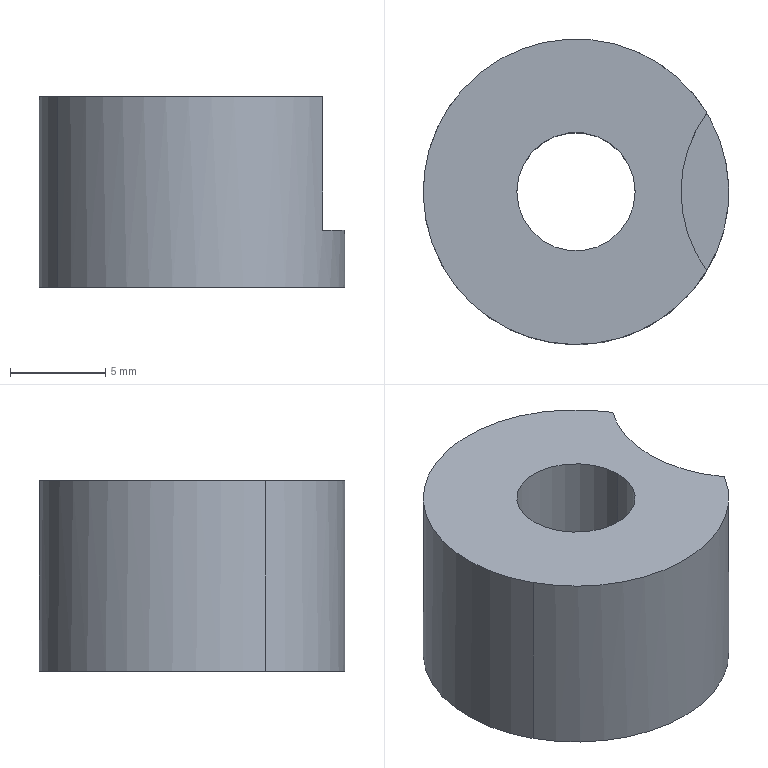Part | CATIA | 1 solid | 9 faces | box 16 x 16 x 10 mm | volume 1611 mm3 | cylinder 6 | plane 3 | commonest cylinder face diameters 6.2 x2 14 x2 16 x2
STEP:
#1=CARTESIAN_POINT('',(-7.021,-3.835,-10.));
#2=VERTEX_POINT('',#1);
#3=CARTESIAN_POINT('',(7.021,3.835,-10.));
#4=VERTEX_POINT('',#3);
#5=CARTESIAN_POINT('',(0.,0.,-10.));
#6=DIRECTION('',(0.,0.,1.));
#7=AXIS2_PLACEMENT_3D('',#5,#6,$);
#8=CIRCLE('',#7,8.);
#9=EDGE_CURVE('',#2,#4,#8,.T.);
#10=ORIENTED_EDGE('',*,*,#9,.F.);
#11=CARTESIAN_POINT('',(0.,0.,-10.));
#12=DIRECTION('',(0.,0.,1.));
#13=AXIS2_PLACEMENT_3D('',#11,#12,$);
#14=CIRCLE('',#13,8.);
#15=EDGE_CURVE('',#4,#2,#14,.T.);
#16=ORIENTED_EDGE('',*,*,#15,.F.);
#17=EDGE_LOOP('',(#10,#16));
#18=FACE_OUTER_BOUND('',#17,.T.);
#19=CARTESIAN_POINT('',(-3.1,0.,-10.));
#20=VERTEX_POINT('',#19);
#21=CARTESIAN_POINT('',(3.1,0.,-10.));
#22=VERTEX_POINT('',#21);
#23=CARTESIAN_POINT('',(0.,0.,-10.));
#24=DIRECTION('',(0.,0.,1.));
#25=AXIS2_PLACEMENT_3D('',#23,#24,$);
#26=CIRCLE('',#25,3.1);
#27=EDGE_CURVE('',#20,#22,#26,.T.);
#28=ORIENTED_EDGE('',*,*,#27,.T.);
#29=CARTESIAN_POINT('',(0.,0.,-10.));
#30=DIRECTION('',(0.,0.,1.));
#31=AXIS2_PLACEMENT_3D('',#29,#30,$);
#32=CIRCLE('',#31,3.1);
#33=EDGE_CURVE('',#22,#20,#32,.T.);
#34=ORIENTED_EDGE('',*,*,#33,.T.);
#35=EDGE_LOOP('',(#28,#34));
#36=FACE_BOUND('',#35,.T.);
#37=CARTESIAN_POINT('',(8.,0.,-10.));
#38=DIRECTION('',(0.,0.,1.));
#39=DIRECTION('',(1.,0.,0.));
#40=AXIS2_PLACEMENT_3D('',#37,#38,#39);
#41=PLANE('',#40);
#42=ADVANCED_FACE('',(#18,#36),#41,.F.);
#43=ORIENTED_EDGE('',*,*,#27,.F.);
#44=CARTESIAN_POINT('',(-3.1,0.,0.));
#45=VERTEX_POINT('',#44);
#46=CARTESIAN_POINT('',(-3.1,0.,-16.61));
#47=DIRECTION('',(0.,0.,-1.));
#48=VECTOR('',#47,1.);
#49=LINE('',#46,#48);
#50=EDGE_CURVE('',#45,#20,#49,.T.);
#51=ORIENTED_EDGE('',*,*,#50,.F.);
#52=CARTESIAN_POINT('',(3.1,0.,0.));
#53=VERTEX_POINT('',#52);
#54=CARTESIAN_POINT('',(0.,0.,0.));
#55=DIRECTION('',(0.,0.,-1.));
#56=AXIS2_PLACEMENT_3D('',#54,#55,$);
#57=CIRCLE('',#56,3.1);
#58=EDGE_CURVE('',#53,#45,#57,.T.);
#59=ORIENTED_EDGE('',*,*,#58,.F.);
#60=CARTESIAN_POINT('',(3.1,0.,-16.61));
#61=DIRECTION('',(0.,0.,-1.));
#62=VECTOR('',#61,1.);
#63=LINE('',#60,#62);
#64=EDGE_CURVE('',#53,#22,#63,.T.);
#65=ORIENTED_EDGE('',*,*,#64,.T.);
#66=EDGE_LOOP('',(#43,#51,#59,#65));
#67=FACE_OUTER_BOUND('',#66,.T.);
#68=CARTESIAN_POINT('',(0.,0.,-16.61));
#69=DIRECTION('',(0.,0.,-1.));
#70=DIRECTION('',(1.,0.,0.));
#71=AXIS2_PLACEMENT_3D('',#68,#69,#70);
#72=CYLINDRICAL_SURFACE('',#71,3.1);
#73=ADVANCED_FACE('',(#67),#72,.F.);
#74=ORIENTED_EDGE('',*,*,#33,.F.);
#75=ORIENTED_EDGE('',*,*,#64,.F.);
#76=CARTESIAN_POINT('',(0.,0.,0.));
#77=DIRECTION('',(0.,0.,-1.));
#78=AXIS2_PLACEMENT_3D('',#76,#77,$);
#79=CIRCLE('',#78,3.1);
#80=EDGE_CURVE('',#45,#53,#79,.T.);
#81=ORIENTED_EDGE('',*,*,#80,.F.);
#82=ORIENTED_EDGE('',*,*,#50,.T.);
#83=EDGE_LOOP('',(#74,#75,#81,#82));
#84=FACE_OUTER_BOUND('',#83,.T.);
#85=CARTESIAN_POINT('',(0.,0.,-16.61));
#86=DIRECTION('',(0.,0.,-1.));
#87=DIRECTION('',(-1.,0.,0.));
#88=AXIS2_PLACEMENT_3D('',#85,#86,#87);
#89=CYLINDRICAL_SURFACE('',#88,3.1);
#90=ADVANCED_FACE('',(#84),#89,.F.);
#91=CARTESIAN_POINT('',(6.85,4.132,0.));
#92=VERTEX_POINT('',#91);
#93=CARTESIAN_POINT('',(-7.021,-3.835,0.));
#94=VERTEX_POINT('',#93);
#95=CARTESIAN_POINT('',(0.,0.,0.));
#96=DIRECTION('',(0.,0.,1.));
#97=AXIS2_PLACEMENT_3D('',#95,#96,$);
#98=CIRCLE('',#97,8.);
#99=EDGE_CURVE('',#92,#94,#98,.T.);
#100=ORIENTED_EDGE('',*,*,#99,.T.);
#101=CARTESIAN_POINT('',(6.85,-4.132,0.));
#102=VERTEX_POINT('',#101);
#103=CARTESIAN_POINT('',(0.,0.,0.));
#104=DIRECTION('',(0.,0.,1.));
#105=AXIS2_PLACEMENT_3D('',#103,#104,$);
#106=CIRCLE('',#105,8.);
#107=EDGE_CURVE('',#94,#102,#106,.T.);
#108=ORIENTED_EDGE('',*,*,#107,.T.);
#109=CARTESIAN_POINT('',(5.5,0.,0.));
#110=VERTEX_POINT('',#109);
#111=CARTESIAN_POINT('',(12.5,0.,0.));
#112=DIRECTION('',(0.,0.,1.));
#113=AXIS2_PLACEMENT_3D('',#111,#112,$);
#114=CIRCLE('',#113,7.);
#115=EDGE_CURVE('',#110,#102,#114,.T.);
#116=ORIENTED_EDGE('',*,*,#115,.F.);
#117=CARTESIAN_POINT('',(12.5,0.,0.));
#118=DIRECTION('',(0.,0.,1.));
#119=AXIS2_PLACEMENT_3D('',#117,#118,$);
#120=CIRCLE('',#119,7.);
#121=EDGE_CURVE('',#92,#110,#120,.T.);
#122=ORIENTED_EDGE('',*,*,#121,.F.);
#123=EDGE_LOOP('',(#100,#108,#116,#122));
#124=FACE_OUTER_BOUND('',#123,.T.);
#125=ORIENTED_EDGE('',*,*,#58,.T.);
#126=ORIENTED_EDGE('',*,*,#80,.T.);
#127=EDGE_LOOP('',(#125,#126));
#128=FACE_BOUND('',#127,.T.);
#129=CARTESIAN_POINT('',(0.,0.,0.));
#130=DIRECTION('',(0.,0.,1.));
#131=DIRECTION('',(1.,0.,0.));
#132=AXIS2_PLACEMENT_3D('',#129,#130,#131);
#133=PLANE('',#132);
#134=ADVANCED_FACE('',(#124,#128),#133,.T.);
#135=ORIENTED_EDGE('',*,*,#107,.F.);
#136=CARTESIAN_POINT('',(-7.021,-3.835,-5.));
#137=DIRECTION('',(0.,0.,1.));
#138=VECTOR('',#137,1.);
#139=LINE('',#136,#138);
#140=EDGE_CURVE('',#2,#94,#139,.T.);
#141=ORIENTED_EDGE('',*,*,#140,.F.);
#142=ORIENTED_EDGE('',*,*,#9,.T.);
#143=CARTESIAN_POINT('',(7.021,3.835,-7.));
#144=VERTEX_POINT('',#143);
#145=CARTESIAN_POINT('',(7.021,3.835,-5.));
#146=DIRECTION('',(0.,0.,1.));
#147=VECTOR('',#146,1.);
#148=LINE('',#145,#147);
#149=EDGE_CURVE('',#4,#144,#148,.T.);
#150=ORIENTED_EDGE('',*,*,#149,.T.);
#151=CARTESIAN_POINT('',(6.85,-4.132,-7.));
#152=VERTEX_POINT('',#151);
#153=CARTESIAN_POINT('',(0.,0.,-7.));
#154=DIRECTION('',(0.,0.,1.));
#155=AXIS2_PLACEMENT_3D('',#153,#154,$);
#156=CIRCLE('',#155,8.);
#157=EDGE_CURVE('',#152,#144,#156,.T.);
#158=ORIENTED_EDGE('',*,*,#157,.F.);
#159=CARTESIAN_POINT('',(6.85,-4.132,-5.));
#160=DIRECTION('',(0.,0.,1.));
#161=VECTOR('',#160,1.);
#162=LINE('',#159,#161);
#163=EDGE_CURVE('',#152,#102,#162,.T.);
#164=ORIENTED_EDGE('',*,*,#163,.T.);
#165=EDGE_LOOP('',(#135,#141,#142,#150,#158,#164));
#166=FACE_OUTER_BOUND('',#165,.T.);
#167=CARTESIAN_POINT('',(0.,0.,-5.));
#168=DIRECTION('',(0.,0.,1.));
#169=DIRECTION('',(0.8776,0.4794,0.));
#170=AXIS2_PLACEMENT_3D('',#167,#168,#169);
#171=CYLINDRICAL_SURFACE('',#170,8.);
#172=ADVANCED_FACE('',(#166),#171,.T.);
#173=ORIENTED_EDGE('',*,*,#149,.F.);
#174=ORIENTED_EDGE('',*,*,#15,.T.);
#175=ORIENTED_EDGE('',*,*,#140,.T.);
#176=ORIENTED_EDGE('',*,*,#99,.F.);
#177=CARTESIAN_POINT('',(6.85,4.132,-7.));
#178=VERTEX_POINT('',#177);
#179=CARTESIAN_POINT('',(6.85,4.132,-5.));
#180=DIRECTION('',(0.,0.,1.));
#181=VECTOR('',#180,1.);
#182=LINE('',#179,#181);
#183=EDGE_CURVE('',#178,#92,#182,.T.);
#184=ORIENTED_EDGE('',*,*,#183,.F.);
#185=CARTESIAN_POINT('',(0.,0.,-7.));
#186=DIRECTION('',(0.,0.,1.));
#187=AXIS2_PLACEMENT_3D('',#185,#186,$);
#188=CIRCLE('',#187,8.);
#189=EDGE_CURVE('',#144,#178,#188,.T.);
#190=ORIENTED_EDGE('',*,*,#189,.F.);
#191=EDGE_LOOP('',(#173,#174,#175,#176,#184,#190));
#192=FACE_OUTER_BOUND('',#191,.T.);
#193=ADVANCED_FACE('',(#192),#171,.T.);
#194=CARTESIAN_POINT('',(5.5,0.,-7.));
#195=VERTEX_POINT('',#194);
#196=CARTESIAN_POINT('',(12.5,0.,-7.));
#197=DIRECTION('',(0.,0.,1.));
#198=AXIS2_PLACEMENT_3D('',#196,#197,$);
#199=CIRCLE('',#198,7.);
#200=EDGE_CURVE('',#178,#195,#199,.T.);
#201=ORIENTED_EDGE('',*,*,#200,.T.);
#202=CARTESIAN_POINT('',(12.5,0.,-7.));
#203=DIRECTION('',(0.,0.,1.));
#204=AXIS2_PLACEMENT_3D('',#202,#203,$);
#205=CIRCLE('',#204,7.);
#206=EDGE_CURVE('',#195,#152,#205,.T.);
#207=ORIENTED_EDGE('',*,*,#206,.T.);
#208=ORIENTED_EDGE('',*,*,#157,.T.);
#209=ORIENTED_EDGE('',*,*,#189,.T.);
#210=EDGE_LOOP('',(#201,#207,#208,#209));
#211=FACE_OUTER_BOUND('',#210,.T.);
#212=CARTESIAN_POINT('',(0.,0.,-7.));
#213=DIRECTION('',(0.,0.,1.));
#214=DIRECTION('',(1.,0.,0.));
#215=AXIS2_PLACEMENT_3D('',#212,#213,#214);
#216=PLANE('',#215);
#217=ADVANCED_FACE('',(#211),#216,.T.);
#218=ORIENTED_EDGE('',*,*,#183,.T.);
#219=ORIENTED_EDGE('',*,*,#121,.T.);
#220=CARTESIAN_POINT('',(5.5,0.,-4.11));
#221=DIRECTION('',(0.,0.,1.));
#222=VECTOR('',#221,1.);
#223=LINE('',#220,#222);
#224=EDGE_CURVE('',#110,#195,#223,.F.);
#225=ORIENTED_EDGE('',*,*,#224,.T.);
#226=ORIENTED_EDGE('',*,*,#200,.F.);
#227=EDGE_LOOP('',(#218,#219,#225,#226));
#228=FACE_OUTER_BOUND('',#227,.T.);
#229=CARTESIAN_POINT('',(12.5,0.,-4.11));
#230=DIRECTION('',(0.,0.,1.));
#231=DIRECTION('',(1.,0.,0.));
#232=AXIS2_PLACEMENT_3D('',#229,#230,#231);
#233=CYLINDRICAL_SURFACE('',#232,7.);
#234=ADVANCED_FACE('',(#228),#233,.F.);
#235=ORIENTED_EDGE('',*,*,#163,.F.);
#236=ORIENTED_EDGE('',*,*,#206,.F.);
#237=ORIENTED_EDGE('',*,*,#224,.F.);
#238=ORIENTED_EDGE('',*,*,#115,.T.);
#239=EDGE_LOOP('',(#235,#236,#237,#238));
#240=FACE_OUTER_BOUND('',#239,.T.);
#241=ADVANCED_FACE('',(#240),#233,.F.);
#242=CLOSED_SHELL('',(#42,#73,#90,#134,#172,#193,#217,#234,#241));
#243=MANIFOLD_SOLID_BREP('',#242);
#244=(LENGTH_UNIT()NAMED_UNIT(*)SI_UNIT(.MILLI.,.METRE.));
#245=UNCERTAINTY_MEASURE_WITH_UNIT(LENGTH_MEASURE(0.005),#244,'','');
#246=(NAMED_UNIT(*)PLANE_ANGLE_UNIT()SI_UNIT($,.RADIAN.));
#247=(NAMED_UNIT(*)SI_UNIT($,.STERADIAN.)SOLID_ANGLE_UNIT());
#248=(GEOMETRIC_REPRESENTATION_CONTEXT(3)GLOBAL_UNCERTAINTY_ASSIGNED_CONTEXT((#245))GLOBAL_UNIT_ASSIGNED_CONTEXT((#244,#246,#247))REPRESENTATION_CONTEXT('',''));
#249=ADVANCED_BREP_SHAPE_REPRESENTATION('',(#243),#248);